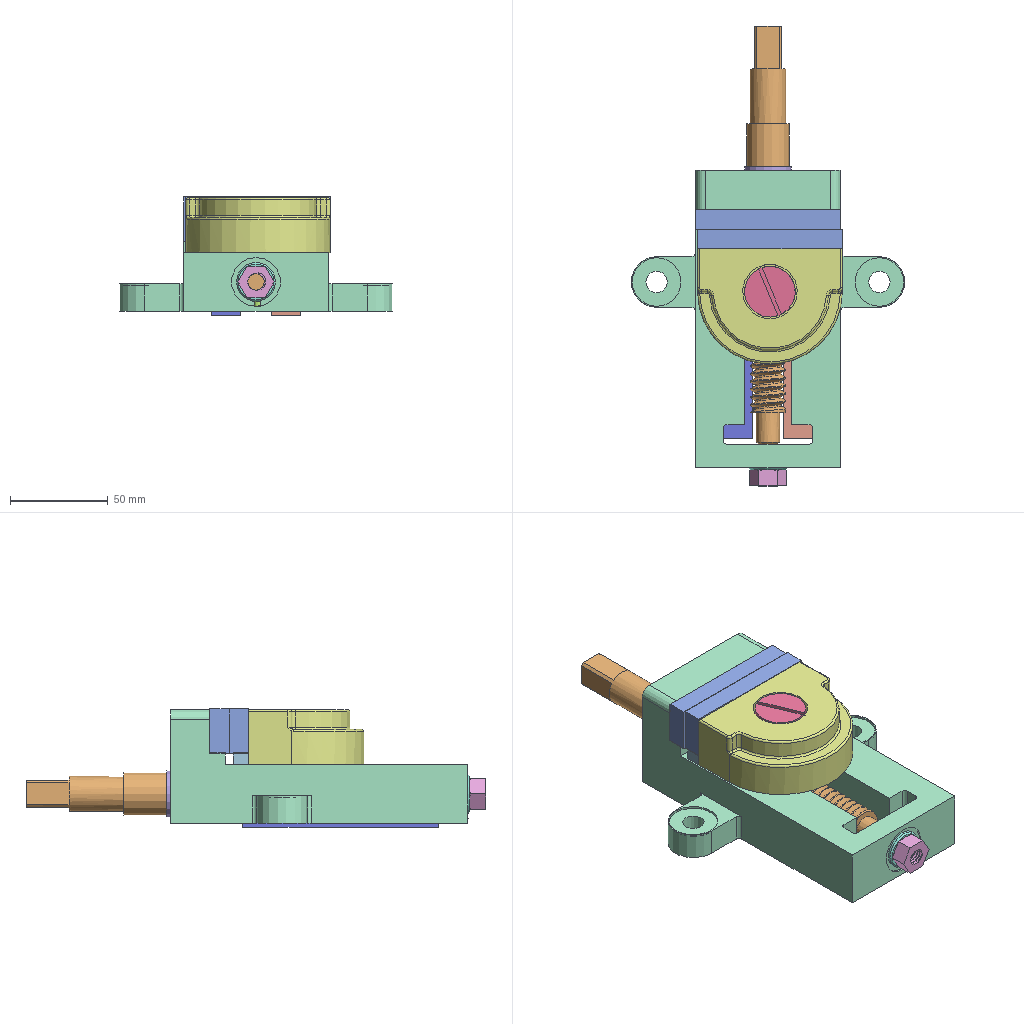Assembly | NX | 11 different items | 15 placed | box 140 x 235 x 60 mm
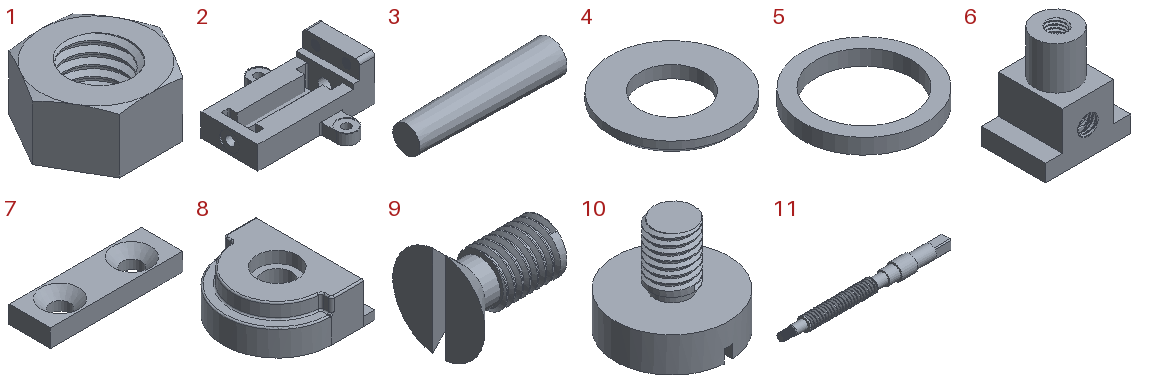Parts list (item | quantity | size | volume | features):
1 | x1 | 18.475 x 16 x 8.4 mm | 1288 mm3 | features CHAMFER 1, CYLINDER 1, DATUM_CSYS 1, EXTRUDE 1, HOLE PACKAGE 1, SIMPLE HOLE 1, THREADS 1
2 | x1 | 152 x 140 x 60 mm | 327609 mm3 | features DATUM_CSYS 11, SKETCH 10, EXTRUDE 8, SIMPLE HOLE 4, HOLE PACKAGE 3, BLEND 2, THREADS 2
3 | x1 | 16 x 3.64 x 3.64 mm | 138.94 mm3 | features DATUM_CSYS 2, SKETCH 1, SWP104 1
4 | x1 | 20 x 20 x 2 mm | 435.568 mm3 | features DATUM_CSYS 2, CHAMFER 1, EXTRUDE 1, SKETCH 1
5 | x1 | 24 x 24 x 3 mm | 550.76 mm3 | features DATUM_CSYS 2, EXTRUDE 1, SKETCH 1
6 | x1 | 40 x 30 x 46 mm | 25067 mm3 | features DATUM_CSYS 3, HOLE PACKAGE 2, SIMPLE HOLE 2, SKETCH 2, THREADS 2, BLOCK 1, CYLINDER 1, EXTRUDE 1, UNITE 1
7 | x2 | 74 x 23 x 10 mm | 13994 mm3 | features DATUM_CSYS 3, CSUNK_HOLE 2, HOLE PACKAGE 2, SKETCH 2, EXTRUDE 1, MIRROR_SET 1
8 | x1 | 67 x 74 x 28 mm | 88703 mm3 | features DATUM_CSYS 6, SKETCH 5, HOLE PACKAGE 3, BLEND 2, EXTRUDE 2, MIRROR_SET 2, SIMPLE HOLE 2, THREADS 2, CBORE_HOLE 1, SKIN 1
9 | x4 | 20 x 18 x 17.826 mm | 1535 mm3 | features DATUM_CSYS 3, SKETCH 2, EXTRUDE 1, SWP104 1, THREADS 1
10 | x1 | 26 x 26 x 22 mm | 4995 mm3 | features CYLINDER 2, DATUM_CSYS 2, EXTRUDE 1, RECT_GROOVE 1, SKETCH 1, THREADS 1
11 | x1 | 230 x 22 x 22 mm | 46800 mm3 | features DATUM_CSYS 4, SKETCH 3, EXTRUDE 2, THREADS 2, CHAMFER 1, SWP104 1
Mates (type | each side: item.copy, entity, surface, feature):
Concentric | 9.1 edge | 7.1 edge | 4 times
Concentric | 7.1 edge | assembly edge
Concentric | 7.1 edge | 8.1 edge
Concentric | 10.1 edge | 8.1 edge
Concentric | 5.1 edge | assembly edge
Concentric | 11.1 edge | 5.1 edge
Concentric | 4.1 edge | assembly edge
Concentric | 1.1 edge | 4.1 edge
Concentric | 6.1 edge | 8.1 edge
Touch | 8.1 face plane Extrude(2) | assembly face plane Extrude(2)
Distance | 7.1 face plane Extrude(2) | 7.1 face plane Extrude(2)